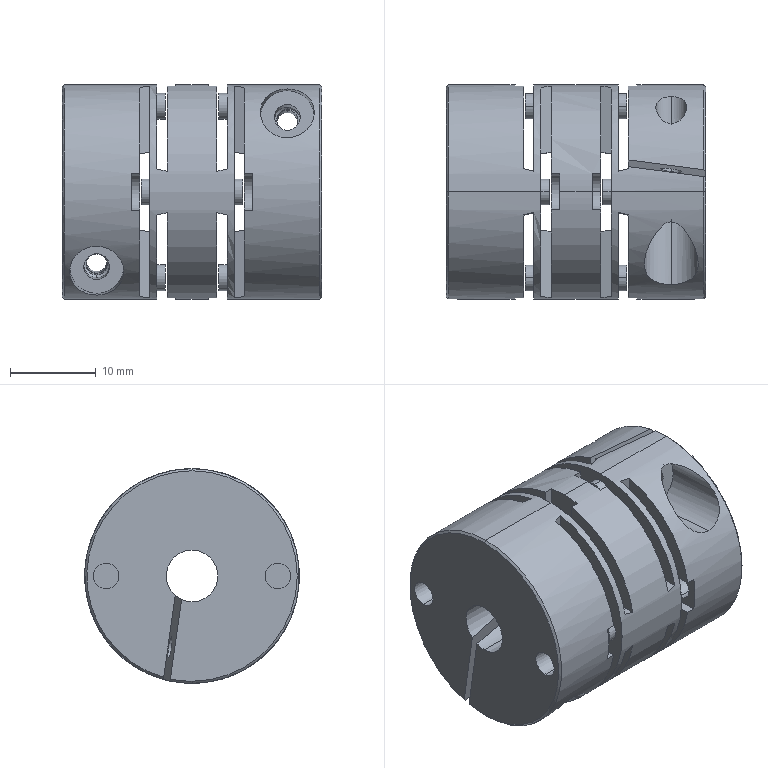Part | NX | features BREP 1 | 1 solid | 153 faces | box 30.2 x 25 x 25 mm | volume 10494 mm3 | plane 74 | cylinder 64 | cone 15 | commonest cylinder face diameters 3 x28 4.2 x10 2.459 x7 3.6 x4 6.3 x4 6 x3